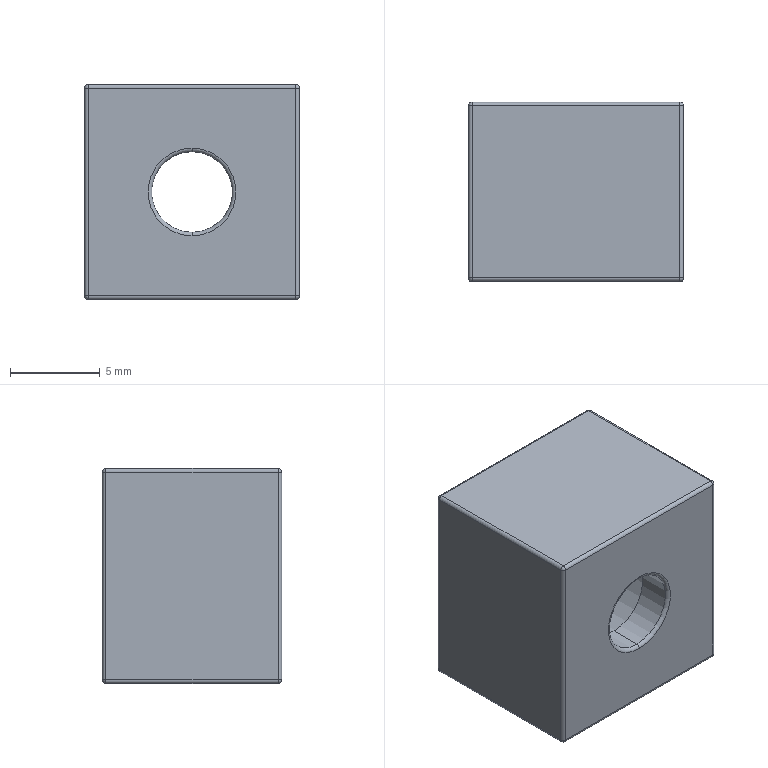Part | STEP file | bumper sleeve 12-M4 | 1 solid | 35 faces | box 12 x 10 x 12 mm | volume 1005 mm3 | cylinder 16 | sphere 8 | plane 7 | torus 4 | commonest cylinder face diameters 0.4 x12 4.5 x2 8 x2